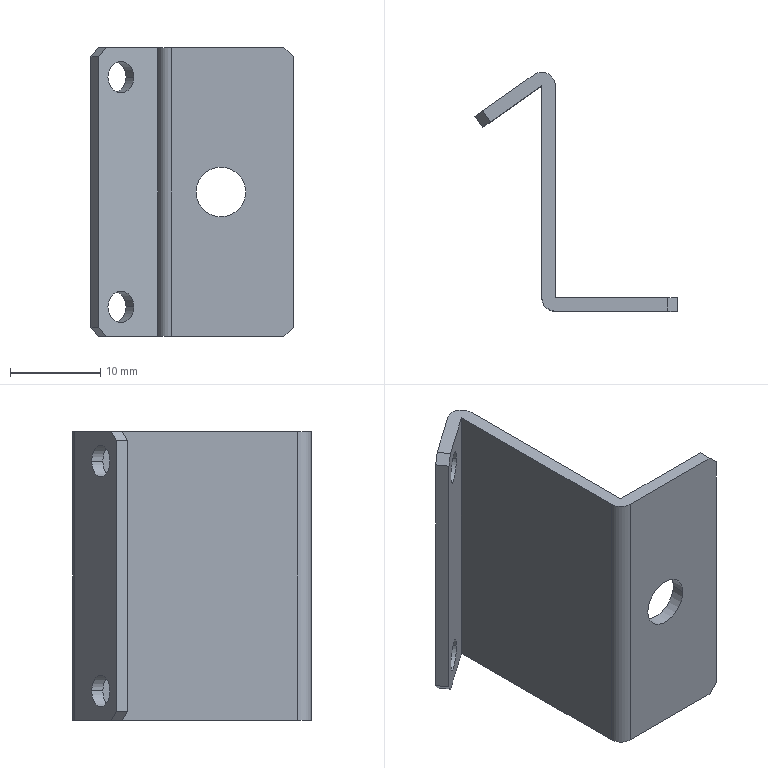Part | STEP file | Photoelectric switch mounting plate | 1 solid | 22 faces | box 22.414 x 26.5 x 32 mm | volume 2228 mm3 | plane 14 | cylinder 8 | commonest cylinder face diameters 3.5 x4 3 x2 5.5 x2